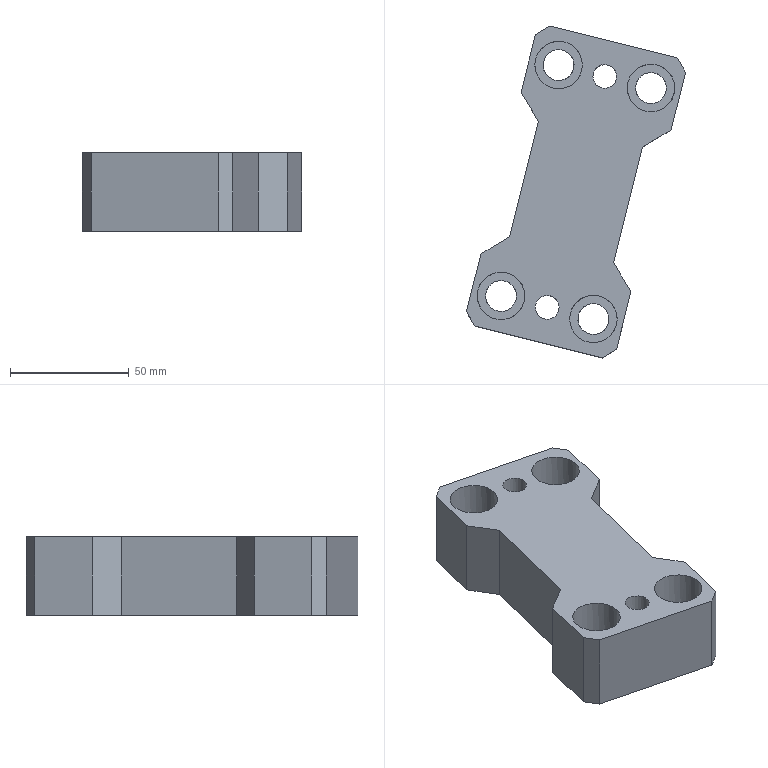Part | NX | features solid 2 | 1 solid | 32 faces | box 92.1 x 139.444 x 33 mm | volume 201833 mm3 | plane 22 | cylinder 10 | commonest cylinder face diameters 13 x4 20 x4 10 x2
STEP:
#1=CARTESIAN_POINT('',(-924.35,446.026,23.));
#2=VERTEX_POINT('',#1);
#3=CARTESIAN_POINT('',(-914.647,443.606,23.));
#4=DIRECTION('',(0.,0.,1.));
#5=DIRECTION('',(-0.9703,0.2419,0.));
#6=AXIS2_PLACEMENT_3D('',#3,#4,#5);
#7=CIRCLE('',#6,10.);
#8=EDGE_CURVE('',#2,#2,#7,.F.);
#9=ORIENTED_EDGE('',*,*,#8,.T.);
#10=EDGE_LOOP('',(#9));
#11=FACE_BOUND('',#10,.T.);
#12=CARTESIAN_POINT('',(-948.542,348.996,23.));
#13=VERTEX_POINT('',#12);
#14=CARTESIAN_POINT('',(-938.839,346.577,23.));
#15=DIRECTION('',(0.,0.,1.));
#16=DIRECTION('',(-0.9703,0.2419,0.));
#17=AXIS2_PLACEMENT_3D('',#14,#15,#16);
#18=CIRCLE('',#17,10.);
#19=EDGE_CURVE('',#13,#13,#18,.F.);
#20=ORIENTED_EDGE('',*,*,#19,.T.);
#21=EDGE_LOOP('',(#20));
#22=FACE_BOUND('',#21,.T.);
#23=CARTESIAN_POINT('',(-900.092,439.978,23.));
#24=VERTEX_POINT('',#23);
#25=CARTESIAN_POINT('',(-895.241,438.768,23.));
#26=DIRECTION('',(0.,0.,1.));
#27=DIRECTION('',(-0.9703,0.2419,0.));
#28=AXIS2_PLACEMENT_3D('',#25,#26,#27);
#29=CIRCLE('',#28,5.);
#30=EDGE_CURVE('',#24,#24,#29,.F.);
#31=ORIENTED_EDGE('',*,*,#30,.T.);
#32=EDGE_LOOP('',(#31));
#33=FACE_BOUND('',#32,.T.);
#34=CARTESIAN_POINT('',(-949.745,333.837,23.));
#35=VERTEX_POINT('',#34);
#36=CARTESIAN_POINT('',(-896.379,320.531,23.));
#37=VERTEX_POINT('',#36);
#38=CARTESIAN_POINT('',(-891.527,319.321,23.));
#39=DIRECTION('',(0.9703,-0.2419,0.));
#40=VECTOR('',#39,1000.);
#41=LINE('',#38,#40);
#42=EDGE_CURVE('',#35,#37,#41,.T.);
#43=ORIENTED_EDGE('',*,*,#42,.T.);
#44=CARTESIAN_POINT('',(-890.318,324.173,23.));
#45=VERTEX_POINT('',#44);
#46=CARTESIAN_POINT('',(-896.379,320.531,23.));
#47=DIRECTION('',(-0.8572,-0.515,0.));
#48=VECTOR('',#47,1000.);
#49=LINE('',#46,#48);
#50=EDGE_CURVE('',#45,#37,#49,.T.);
#51=ORIENTED_EDGE('',*,*,#50,.F.);
#52=CARTESIAN_POINT('',(-884.27,348.43,23.));
#53=VERTEX_POINT('',#52);
#54=CARTESIAN_POINT('',(-891.527,319.321,23.));
#55=DIRECTION('',(-0.2419,-0.9703,0.));
#56=VECTOR('',#55,1000.);
#57=LINE('',#54,#56);
#58=EDGE_CURVE('',#53,#45,#57,.T.);
#59=ORIENTED_EDGE('',*,*,#58,.F.);
#60=CARTESIAN_POINT('',(-891.553,360.553,23.));
#61=VERTEX_POINT('',#60);
#62=CARTESIAN_POINT('',(-873.344,330.247,23.));
#63=DIRECTION('',(0.515,-0.8572,0.));
#64=VECTOR('',#63,1000.);
#65=LINE('',#62,#64);
#66=EDGE_CURVE('',#61,#53,#65,.T.);
#67=ORIENTED_EDGE('',*,*,#66,.F.);
#68=CARTESIAN_POINT('',(-879.457,409.067,23.));
#69=VERTEX_POINT('',#68);
#70=CARTESIAN_POINT('',(-901.23,321.741,23.));
#71=DIRECTION('',(-0.2419,-0.9703,0.));
#72=VECTOR('',#71,1000.);
#73=LINE('',#70,#72);
#74=EDGE_CURVE('',#69,#61,#73,.T.);
#75=ORIENTED_EDGE('',*,*,#74,.F.);
#76=CARTESIAN_POINT('',(-867.335,416.351,23.));
#77=VERTEX_POINT('',#76);
#78=CARTESIAN_POINT('',(-927.946,379.932,23.));
#79=DIRECTION('',(0.8572,0.515,0.));
#80=VECTOR('',#79,1000.);
#81=LINE('',#78,#80);
#82=EDGE_CURVE('',#69,#77,#81,.T.);
#83=ORIENTED_EDGE('',*,*,#82,.T.);
#84=CARTESIAN_POINT('',(-861.287,440.608,23.));
#85=VERTEX_POINT('',#84);
#86=CARTESIAN_POINT('',(-891.527,319.321,23.));
#87=DIRECTION('',(-0.2419,-0.9703,0.));
#88=VECTOR('',#87,1000.);
#89=LINE('',#86,#88);
#90=EDGE_CURVE('',#85,#77,#89,.T.);
#91=ORIENTED_EDGE('',*,*,#90,.F.);
#92=CARTESIAN_POINT('',(-864.929,446.67,23.));
#93=VERTEX_POINT('',#92);
#94=CARTESIAN_POINT('',(-861.287,440.608,23.));
#95=DIRECTION('',(-0.515,0.8572,0.));
#96=VECTOR('',#95,1000.);
#97=LINE('',#94,#96);
#98=EDGE_CURVE('',#93,#85,#97,.F.);
#99=ORIENTED_EDGE('',*,*,#98,.F.);
#100=CARTESIAN_POINT('',(-918.295,459.975,23.));
#101=VERTEX_POINT('',#100);
#102=CARTESIAN_POINT('',(-860.077,445.46,23.));
#103=DIRECTION('',(0.9703,-0.2419,0.));
#104=VECTOR('',#103,1000.);
#105=LINE('',#102,#104);
#106=EDGE_CURVE('',#101,#93,#105,.T.);
#107=ORIENTED_EDGE('',*,*,#106,.F.);
#108=CARTESIAN_POINT('',(-924.356,456.333,23.));
#109=VERTEX_POINT('',#108);
#110=CARTESIAN_POINT('',(-918.295,459.975,23.));
#111=DIRECTION('',(0.8572,0.515,0.));
#112=VECTOR('',#111,1000.);
#113=LINE('',#110,#112);
#114=EDGE_CURVE('',#109,#101,#113,.T.);
#115=ORIENTED_EDGE('',*,*,#114,.F.);
#116=CARTESIAN_POINT('',(-930.404,432.076,23.));
#117=VERTEX_POINT('',#116);
#118=CARTESIAN_POINT('',(-954.596,335.046,23.));
#119=DIRECTION('',(-0.2419,-0.9703,0.));
#120=VECTOR('',#119,1000.);
#121=LINE('',#118,#120);
#122=EDGE_CURVE('',#109,#117,#121,.T.);
#123=ORIENTED_EDGE('',*,*,#122,.T.);
#124=CARTESIAN_POINT('',(-923.12,419.954,23.));
#125=VERTEX_POINT('',#124);
#126=CARTESIAN_POINT('',(-870.313,332.068,23.));
#127=DIRECTION('',(0.515,-0.8572,0.));
#128=VECTOR('',#127,1000.);
#129=LINE('',#126,#128);
#130=EDGE_CURVE('',#117,#125,#129,.T.);
#131=ORIENTED_EDGE('',*,*,#130,.T.);
#132=CARTESIAN_POINT('',(-935.217,371.439,23.));
#133=VERTEX_POINT('',#132);
#134=CARTESIAN_POINT('',(-944.893,332.627,23.));
#135=DIRECTION('',(-0.2419,-0.9703,0.));
#136=VECTOR('',#135,1000.);
#137=LINE('',#134,#136);
#138=EDGE_CURVE('',#125,#133,#137,.T.);
#139=ORIENTED_EDGE('',*,*,#138,.T.);
#140=CARTESIAN_POINT('',(-947.339,364.155,23.));
#141=VERTEX_POINT('',#140);
#142=CARTESIAN_POINT('',(-926.125,376.902,23.));
#143=DIRECTION('',(0.8572,0.515,0.));
#144=VECTOR('',#143,1000.);
#145=LINE('',#142,#144);
#146=EDGE_CURVE('',#141,#133,#145,.T.);
#147=ORIENTED_EDGE('',*,*,#146,.F.);
#148=CARTESIAN_POINT('',(-953.387,339.898,23.));
#149=VERTEX_POINT('',#148);
#150=CARTESIAN_POINT('',(-954.596,335.046,23.));
#151=DIRECTION('',(-0.2419,-0.9703,0.));
#152=VECTOR('',#151,1000.);
#153=LINE('',#150,#152);
#154=EDGE_CURVE('',#141,#149,#153,.T.);
#155=ORIENTED_EDGE('',*,*,#154,.T.);
#156=CARTESIAN_POINT('',(-953.387,339.898,23.));
#157=DIRECTION('',(0.515,-0.8572,0.));
#158=VECTOR('',#157,1000.);
#159=LINE('',#156,#158);
#160=EDGE_CURVE('',#35,#149,#159,.F.);
#161=ORIENTED_EDGE('',*,*,#160,.F.);
#162=EDGE_LOOP('',(#43,#51,#59,#67,#75,#83,#91,#99,#107,#115,#123,#131,#139,#147,#155,#161));
#163=FACE_BOUND('',#162,.T.);
#164=CARTESIAN_POINT('',(-924.284,342.948,23.));
#165=VERTEX_POINT('',#164);
#166=CARTESIAN_POINT('',(-919.433,341.738,23.));
#167=DIRECTION('',(0.,0.,1.));
#168=DIRECTION('',(-0.9703,0.2419,0.));
#169=AXIS2_PLACEMENT_3D('',#166,#167,#168);
#170=CIRCLE('',#169,5.);
#171=EDGE_CURVE('',#165,#165,#170,.F.);
#172=ORIENTED_EDGE('',*,*,#171,.T.);
#173=EDGE_LOOP('',(#172));
#174=FACE_BOUND('',#173,.T.);
#175=CARTESIAN_POINT('',(-909.73,339.319,23.));
#176=VERTEX_POINT('',#175);
#177=CARTESIAN_POINT('',(-900.027,336.9,23.));
#178=DIRECTION('',(0.,0.,1.));
#179=DIRECTION('',(-0.9703,0.2419,0.));
#180=AXIS2_PLACEMENT_3D('',#177,#178,#179);
#181=CIRCLE('',#180,10.);
#182=EDGE_CURVE('',#176,#176,#181,.F.);
#183=ORIENTED_EDGE('',*,*,#182,.T.);
#184=EDGE_LOOP('',(#183));
#185=FACE_BOUND('',#184,.T.);
#186=CARTESIAN_POINT('',(-885.538,436.349,23.));
#187=VERTEX_POINT('',#186);
#188=CARTESIAN_POINT('',(-875.835,433.93,23.));
#189=DIRECTION('',(0.,0.,1.));
#190=DIRECTION('',(-0.9703,0.2419,0.));
#191=AXIS2_PLACEMENT_3D('',#188,#189,#190);
#192=CIRCLE('',#191,10.);
#193=EDGE_CURVE('',#187,#187,#192,.F.);
#194=ORIENTED_EDGE('',*,*,#193,.T.);
#195=EDGE_LOOP('',(#194));
#196=FACE_BOUND('',#195,.T.);
#197=CARTESIAN_POINT('',(-891.527,319.321,23.));
#198=DIRECTION('',(0.,0.,-1.));
#199=DIRECTION('',(-0.9703,0.2419,0.));
#200=AXIS2_PLACEMENT_3D('',#197,#198,#199);
#201=PLANE('',#200);
#202=ADVANCED_FACE('',(#11,#22,#33,#163,#174,#185,#196),#201,.F.);
#203=CARTESIAN_POINT('',(-877.407,427.623,-10.));
#204=VERTEX_POINT('',#203);
#205=CARTESIAN_POINT('',(-875.835,433.93,-10.));
#206=DIRECTION('',(0.,0.,-1.));
#207=DIRECTION('',(-0.2419,-0.9703,0.));
#208=AXIS2_PLACEMENT_3D('',#205,#206,#207);
#209=CIRCLE('',#208,6.5);
#210=EDGE_CURVE('',#204,#204,#209,.T.);
#211=ORIENTED_EDGE('',*,*,#210,.T.);
#212=EDGE_LOOP('',(#211));
#213=FACE_BOUND('',#212,.T.);
#214=CARTESIAN_POINT('',(-869.528,432.357,5.));
#215=VERTEX_POINT('',#214);
#216=CARTESIAN_POINT('',(-875.835,433.93,5.));
#217=DIRECTION('',(0.,0.,-1.));
#218=DIRECTION('',(0.9703,-0.2419,0.));
#219=AXIS2_PLACEMENT_3D('',#216,#217,#218);
#220=CIRCLE('',#219,6.5);
#221=EDGE_CURVE('',#215,#215,#220,.T.);
#222=ORIENTED_EDGE('',*,*,#221,.F.);
#223=EDGE_LOOP('',(#222));
#224=FACE_BOUND('',#223,.T.);
#225=CARTESIAN_POINT('',(-875.835,433.93,12.));
#226=DIRECTION('',(0.,0.,-1.));
#227=DIRECTION('',(-0.9703,0.2419,0.));
#228=AXIS2_PLACEMENT_3D('',#225,#226,#227);
#229=CYLINDRICAL_SURFACE('',#228,6.5);
#230=ADVANCED_FACE('',(#213,#224),#229,.F.);
#231=CARTESIAN_POINT('',(-916.219,437.299,-10.));
#232=VERTEX_POINT('',#231);
#233=CARTESIAN_POINT('',(-914.647,443.606,-10.));
#234=DIRECTION('',(0.,0.,-1.));
#235=DIRECTION('',(-0.2419,-0.9703,0.));
#236=AXIS2_PLACEMENT_3D('',#233,#234,#235);
#237=CIRCLE('',#236,6.5);
#238=EDGE_CURVE('',#232,#232,#237,.T.);
#239=ORIENTED_EDGE('',*,*,#238,.T.);
#240=EDGE_LOOP('',(#239));
#241=FACE_BOUND('',#240,.T.);
#242=CARTESIAN_POINT('',(-908.34,442.034,5.));
#243=VERTEX_POINT('',#242);
#244=CARTESIAN_POINT('',(-914.647,443.606,5.));
#245=DIRECTION('',(0.,0.,-1.));
#246=DIRECTION('',(0.9703,-0.2419,0.));
#247=AXIS2_PLACEMENT_3D('',#244,#245,#246);
#248=CIRCLE('',#247,6.5);
#249=EDGE_CURVE('',#243,#243,#248,.T.);
#250=ORIENTED_EDGE('',*,*,#249,.F.);
#251=EDGE_LOOP('',(#250));
#252=FACE_BOUND('',#251,.T.);
#253=CARTESIAN_POINT('',(-914.647,443.606,12.));
#254=DIRECTION('',(0.,0.,-1.));
#255=DIRECTION('',(-0.9703,0.2419,0.));
#256=AXIS2_PLACEMENT_3D('',#253,#254,#255);
#257=CYLINDRICAL_SURFACE('',#256,6.5);
#258=ADVANCED_FACE('',(#241,#252),#257,.F.);
#259=CARTESIAN_POINT('',(-901.6,330.593,-10.));
#260=VERTEX_POINT('',#259);
#261=CARTESIAN_POINT('',(-900.027,336.9,-10.));
#262=DIRECTION('',(0.,0.,-1.));
#263=DIRECTION('',(-0.2419,-0.9703,0.));
#264=AXIS2_PLACEMENT_3D('',#261,#262,#263);
#265=CIRCLE('',#264,6.5);
#266=EDGE_CURVE('',#260,#260,#265,.T.);
#267=ORIENTED_EDGE('',*,*,#266,.T.);
#268=EDGE_LOOP('',(#267));
#269=FACE_BOUND('',#268,.T.);
#270=CARTESIAN_POINT('',(-893.72,335.327,5.));
#271=VERTEX_POINT('',#270);
#272=CARTESIAN_POINT('',(-900.027,336.9,5.));
#273=DIRECTION('',(0.,0.,-1.));
#274=DIRECTION('',(0.9703,-0.2419,0.));
#275=AXIS2_PLACEMENT_3D('',#272,#273,#274);
#276=CIRCLE('',#275,6.5);
#277=EDGE_CURVE('',#271,#271,#276,.T.);
#278=ORIENTED_EDGE('',*,*,#277,.F.);
#279=EDGE_LOOP('',(#278));
#280=FACE_BOUND('',#279,.T.);
#281=CARTESIAN_POINT('',(-900.027,336.9,12.));
#282=DIRECTION('',(0.,0.,-1.));
#283=DIRECTION('',(-0.9703,0.2419,0.));
#284=AXIS2_PLACEMENT_3D('',#281,#282,#283);
#285=CYLINDRICAL_SURFACE('',#284,6.5);
#286=ADVANCED_FACE('',(#269,#280),#285,.F.);
#287=CARTESIAN_POINT('',(-940.411,340.27,-10.));
#288=VERTEX_POINT('',#287);
#289=CARTESIAN_POINT('',(-938.839,346.577,-10.));
#290=DIRECTION('',(0.,0.,-1.));
#291=DIRECTION('',(-0.2419,-0.9703,0.));
#292=AXIS2_PLACEMENT_3D('',#289,#290,#291);
#293=CIRCLE('',#292,6.5);
#294=EDGE_CURVE('',#288,#288,#293,.T.);
#295=ORIENTED_EDGE('',*,*,#294,.T.);
#296=EDGE_LOOP('',(#295));
#297=FACE_BOUND('',#296,.T.);
#298=CARTESIAN_POINT('',(-932.532,345.004,5.));
#299=VERTEX_POINT('',#298);
#300=CARTESIAN_POINT('',(-938.839,346.577,5.));
#301=DIRECTION('',(0.,0.,-1.));
#302=DIRECTION('',(0.9703,-0.2419,0.));
#303=AXIS2_PLACEMENT_3D('',#300,#301,#302);
#304=CIRCLE('',#303,6.5);
#305=EDGE_CURVE('',#299,#299,#304,.T.);
#306=ORIENTED_EDGE('',*,*,#305,.F.);
#307=EDGE_LOOP('',(#306));
#308=FACE_BOUND('',#307,.T.);
#309=CARTESIAN_POINT('',(-938.839,346.577,12.));
#310=DIRECTION('',(0.,0.,-1.));
#311=DIRECTION('',(-0.9703,0.2419,0.));
#312=AXIS2_PLACEMENT_3D('',#309,#310,#311);
#313=CYLINDRICAL_SURFACE('',#312,6.5);
#314=ADVANCED_FACE('',(#297,#308),#313,.F.);
#315=CARTESIAN_POINT('',(-896.45,433.916,-10.));
#316=VERTEX_POINT('',#315);
#317=CARTESIAN_POINT('',(-895.241,438.768,-10.));
#318=DIRECTION('',(0.,0.,-1.));
#319=DIRECTION('',(-0.2419,-0.9703,0.));
#320=AXIS2_PLACEMENT_3D('',#317,#318,#319);
#321=CIRCLE('',#320,5.);
#322=EDGE_CURVE('',#316,#316,#321,.T.);
#323=ORIENTED_EDGE('',*,*,#322,.F.);
#324=EDGE_LOOP('',(#323));
#325=FACE_BOUND('',#324,.T.);
#326=ORIENTED_EDGE('',*,*,#266,.F.);
#327=EDGE_LOOP('',(#326));
#328=FACE_BOUND('',#327,.T.);
#329=ORIENTED_EDGE('',*,*,#294,.F.);
#330=EDGE_LOOP('',(#329));
#331=FACE_BOUND('',#330,.T.);
#332=CARTESIAN_POINT('',(-947.339,364.155,-10.));
#333=VERTEX_POINT('',#332);
#334=CARTESIAN_POINT('',(-953.387,339.898,-10.));
#335=VERTEX_POINT('',#334);
#336=CARTESIAN_POINT('',(-947.339,364.155,-10.));
#337=DIRECTION('',(-0.2419,-0.9703,0.));
#338=VECTOR('',#337,1000.);
#339=LINE('',#336,#338);
#340=EDGE_CURVE('',#333,#335,#339,.T.);
#341=ORIENTED_EDGE('',*,*,#340,.F.);
#342=CARTESIAN_POINT('',(-935.217,371.439,-10.));
#343=VERTEX_POINT('',#342);
#344=CARTESIAN_POINT('',(-947.339,364.155,-10.));
#345=DIRECTION('',(0.8572,0.515,0.));
#346=VECTOR('',#345,1000.);
#347=LINE('',#344,#346);
#348=EDGE_CURVE('',#333,#343,#347,.T.);
#349=ORIENTED_EDGE('',*,*,#348,.T.);
#350=CARTESIAN_POINT('',(-923.12,419.954,-10.));
#351=VERTEX_POINT('',#350);
#352=CARTESIAN_POINT('',(-923.12,419.954,-10.));
#353=DIRECTION('',(-0.2419,-0.9703,0.));
#354=VECTOR('',#353,1000.);
#355=LINE('',#352,#354);
#356=EDGE_CURVE('',#351,#343,#355,.T.);
#357=ORIENTED_EDGE('',*,*,#356,.F.);
#358=CARTESIAN_POINT('',(-930.404,432.076,-10.));
#359=VERTEX_POINT('',#358);
#360=CARTESIAN_POINT('',(-930.404,432.076,-10.));
#361=DIRECTION('',(0.515,-0.8572,0.));
#362=VECTOR('',#361,1000.);
#363=LINE('',#360,#362);
#364=EDGE_CURVE('',#359,#351,#363,.T.);
#365=ORIENTED_EDGE('',*,*,#364,.F.);
#366=CARTESIAN_POINT('',(-924.356,456.333,-10.));
#367=VERTEX_POINT('',#366);
#368=CARTESIAN_POINT('',(-923.147,461.185,-10.));
#369=DIRECTION('',(-0.2419,-0.9703,0.));
#370=VECTOR('',#369,1000.);
#371=LINE('',#368,#370);
#372=EDGE_CURVE('',#367,#359,#371,.T.);
#373=ORIENTED_EDGE('',*,*,#372,.F.);
#374=CARTESIAN_POINT('',(-918.295,459.975,-10.));
#375=VERTEX_POINT('',#374);
#376=CARTESIAN_POINT('',(-960.723,434.482,-10.));
#377=DIRECTION('',(-0.8572,-0.515,0.));
#378=VECTOR('',#377,1000.);
#379=LINE('',#376,#378);
#380=EDGE_CURVE('',#375,#367,#379,.T.);
#381=ORIENTED_EDGE('',*,*,#380,.F.);
#382=CARTESIAN_POINT('',(-864.929,446.67,-10.));
#383=VERTEX_POINT('',#382);
#384=CARTESIAN_POINT('',(-923.147,461.185,-10.));
#385=DIRECTION('',(0.9703,-0.2419,0.));
#386=VECTOR('',#385,1000.);
#387=LINE('',#384,#386);
#388=EDGE_CURVE('',#375,#383,#387,.T.);
#389=ORIENTED_EDGE('',*,*,#388,.T.);
#390=CARTESIAN_POINT('',(-861.287,440.608,-10.));
#391=VERTEX_POINT('',#390);
#392=CARTESIAN_POINT('',(-815.764,364.845,-10.));
#393=DIRECTION('',(0.515,-0.8572,0.));
#394=VECTOR('',#393,1000.);
#395=LINE('',#392,#394);
#396=EDGE_CURVE('',#391,#383,#395,.F.);
#397=ORIENTED_EDGE('',*,*,#396,.F.);
#398=CARTESIAN_POINT('',(-867.335,416.351,-10.));
#399=VERTEX_POINT('',#398);
#400=CARTESIAN_POINT('',(-860.077,445.46,-10.));
#401=DIRECTION('',(-0.2419,-0.9703,0.));
#402=VECTOR('',#401,1000.);
#403=LINE('',#400,#402);
#404=EDGE_CURVE('',#391,#399,#403,.T.);
#405=ORIENTED_EDGE('',*,*,#404,.T.);
#406=CARTESIAN_POINT('',(-879.457,409.067,-10.));
#407=VERTEX_POINT('',#406);
#408=CARTESIAN_POINT('',(-879.457,409.067,-10.));
#409=DIRECTION('',(0.8572,0.515,0.));
#410=VECTOR('',#409,1000.);
#411=LINE('',#408,#410);
#412=EDGE_CURVE('',#407,#399,#411,.T.);
#413=ORIENTED_EDGE('',*,*,#412,.F.);
#414=CARTESIAN_POINT('',(-891.553,360.553,-10.));
#415=VERTEX_POINT('',#414);
#416=CARTESIAN_POINT('',(-879.457,409.067,-10.));
#417=DIRECTION('',(-0.2419,-0.9703,0.));
#418=VECTOR('',#417,1000.);
#419=LINE('',#416,#418);
#420=EDGE_CURVE('',#407,#415,#419,.T.);
#421=ORIENTED_EDGE('',*,*,#420,.T.);
#422=CARTESIAN_POINT('',(-884.27,348.43,-10.));
#423=VERTEX_POINT('',#422);
#424=CARTESIAN_POINT('',(-891.553,360.553,-10.));
#425=DIRECTION('',(0.515,-0.8572,0.));
#426=VECTOR('',#425,1000.);
#427=LINE('',#424,#426);
#428=EDGE_CURVE('',#415,#423,#427,.T.);
#429=ORIENTED_EDGE('',*,*,#428,.T.);
#430=CARTESIAN_POINT('',(-890.318,324.173,-10.));
#431=VERTEX_POINT('',#430);
#432=CARTESIAN_POINT('',(-884.27,348.43,-10.));
#433=DIRECTION('',(-0.2419,-0.9703,0.));
#434=VECTOR('',#433,1000.);
#435=LINE('',#432,#434);
#436=EDGE_CURVE('',#423,#431,#435,.T.);
#437=ORIENTED_EDGE('',*,*,#436,.T.);
#438=CARTESIAN_POINT('',(-896.379,320.531,-10.));
#439=VERTEX_POINT('',#438);
#440=CARTESIAN_POINT('',(-893.348,322.352,-10.));
#441=DIRECTION('',(0.8572,0.515,0.));
#442=VECTOR('',#441,1000.);
#443=LINE('',#440,#442);
#444=EDGE_CURVE('',#439,#431,#443,.T.);
#445=ORIENTED_EDGE('',*,*,#444,.F.);
#446=CARTESIAN_POINT('',(-949.745,333.837,-10.));
#447=VERTEX_POINT('',#446);
#448=CARTESIAN_POINT('',(-954.596,335.046,-10.));
#449=DIRECTION('',(0.9703,-0.2419,0.));
#450=VECTOR('',#449,1000.);
#451=LINE('',#448,#450);
#452=EDGE_CURVE('',#447,#439,#451,.T.);
#453=ORIENTED_EDGE('',*,*,#452,.F.);
#454=CARTESIAN_POINT('',(-927.894,297.47,-10.));
#455=DIRECTION('',(-0.515,0.8572,0.));
#456=VECTOR('',#455,1000.);
#457=LINE('',#454,#456);
#458=EDGE_CURVE('',#335,#447,#457,.F.);
#459=ORIENTED_EDGE('',*,*,#458,.F.);
#460=EDGE_LOOP('',(#341,#349,#357,#365,#373,#381,#389,#397,#405,#413,#421,#429,#437,#445,#453,#459));
#461=FACE_BOUND('',#460,.T.);
#462=CARTESIAN_POINT('',(-920.643,336.887,-10.));
#463=VERTEX_POINT('',#462);
#464=CARTESIAN_POINT('',(-919.433,341.738,-10.));
#465=DIRECTION('',(0.,0.,-1.));
#466=DIRECTION('',(-0.2419,-0.9703,0.));
#467=AXIS2_PLACEMENT_3D('',#464,#465,#466);
#468=CIRCLE('',#467,5.);
#469=EDGE_CURVE('',#463,#463,#468,.T.);
#470=ORIENTED_EDGE('',*,*,#469,.F.);
#471=EDGE_LOOP('',(#470));
#472=FACE_BOUND('',#471,.T.);
#473=ORIENTED_EDGE('',*,*,#238,.F.);
#474=EDGE_LOOP('',(#473));
#475=FACE_BOUND('',#474,.T.);
#476=ORIENTED_EDGE('',*,*,#210,.F.);
#477=EDGE_LOOP('',(#476));
#478=FACE_BOUND('',#477,.T.);
#479=CARTESIAN_POINT('',(-891.527,319.321,-10.));
#480=DIRECTION('',(0.,0.,-1.));
#481=DIRECTION('',(-0.9703,0.2419,0.));
#482=AXIS2_PLACEMENT_3D('',#479,#480,#481);
#483=PLANE('',#482);
#484=ADVANCED_FACE('',(#325,#328,#331,#461,#472,#475,#478),#483,.T.);
#485=ORIENTED_EDGE('',*,*,#90,.T.);
#486=CARTESIAN_POINT('',(-867.335,416.351,12.));
#487=DIRECTION('',(0.,0.,-1.));
#488=VECTOR('',#487,1000.);
#489=LINE('',#486,#488);
#490=EDGE_CURVE('',#77,#399,#489,.T.);
#491=ORIENTED_EDGE('',*,*,#490,.T.);
#492=ORIENTED_EDGE('',*,*,#404,.F.);
#493=CARTESIAN_POINT('',(-861.287,440.608,12.));
#494=DIRECTION('',(0.,0.,-1.));
#495=VECTOR('',#494,1000.);
#496=LINE('',#493,#495);
#497=EDGE_CURVE('',#85,#391,#496,.T.);
#498=ORIENTED_EDGE('',*,*,#497,.F.);
#499=EDGE_LOOP('',(#485,#491,#492,#498));
#500=FACE_BOUND('',#499,.T.);
#501=CARTESIAN_POINT('',(-860.077,445.46,12.));
#502=DIRECTION('',(-0.9703,0.2419,0.));
#503=DIRECTION('',(0.2419,0.9703,0.));
#504=AXIS2_PLACEMENT_3D('',#501,#502,#503);
#505=PLANE('',#504);
#506=ADVANCED_FACE('',(#500),#505,.F.);
#507=ORIENTED_EDGE('',*,*,#412,.T.);
#508=ORIENTED_EDGE('',*,*,#490,.F.);
#509=ORIENTED_EDGE('',*,*,#82,.F.);
#510=CARTESIAN_POINT('',(-879.457,409.067,12.));
#511=DIRECTION('',(0.,0.,-1.));
#512=VECTOR('',#511,1000.);
#513=LINE('',#510,#512);
#514=EDGE_CURVE('',#69,#407,#513,.T.);
#515=ORIENTED_EDGE('',*,*,#514,.T.);
#516=EDGE_LOOP('',(#507,#508,#509,#515));
#517=FACE_BOUND('',#516,.T.);
#518=CARTESIAN_POINT('',(-879.457,409.067,12.));
#519=DIRECTION('',(0.515,-0.8572,0.));
#520=DIRECTION('',(-0.8572,-0.515,0.));
#521=AXIS2_PLACEMENT_3D('',#518,#519,#520);
#522=PLANE('',#521);
#523=ADVANCED_FACE('',(#517),#522,.T.);
#524=ORIENTED_EDGE('',*,*,#420,.F.);
#525=ORIENTED_EDGE('',*,*,#514,.F.);
#526=ORIENTED_EDGE('',*,*,#74,.T.);
#527=CARTESIAN_POINT('',(-891.553,360.553,12.));
#528=DIRECTION('',(0.,0.,-1.));
#529=VECTOR('',#528,1000.);
#530=LINE('',#527,#529);
#531=EDGE_CURVE('',#61,#415,#530,.T.);
#532=ORIENTED_EDGE('',*,*,#531,.T.);
#533=EDGE_LOOP('',(#524,#525,#526,#532));
#534=FACE_BOUND('',#533,.T.);
#535=CARTESIAN_POINT('',(-879.457,409.067,12.));
#536=DIRECTION('',(-0.9703,0.2419,0.));
#537=DIRECTION('',(0.2419,0.9703,0.));
#538=AXIS2_PLACEMENT_3D('',#535,#536,#537);
#539=PLANE('',#538);
#540=ADVANCED_FACE('',(#534),#539,.F.);
#541=ORIENTED_EDGE('',*,*,#428,.F.);
#542=ORIENTED_EDGE('',*,*,#531,.F.);
#543=ORIENTED_EDGE('',*,*,#66,.T.);
#544=CARTESIAN_POINT('',(-884.27,348.43,12.));
#545=DIRECTION('',(0.,0.,-1.));
#546=VECTOR('',#545,1000.);
#547=LINE('',#544,#546);
#548=EDGE_CURVE('',#53,#423,#547,.T.);
#549=ORIENTED_EDGE('',*,*,#548,.T.);
#550=EDGE_LOOP('',(#541,#542,#543,#549));
#551=FACE_BOUND('',#550,.T.);
#552=CARTESIAN_POINT('',(-891.553,360.553,12.));
#553=DIRECTION('',(-0.8572,-0.515,0.));
#554=DIRECTION('',(-0.515,0.8572,0.));
#555=AXIS2_PLACEMENT_3D('',#552,#553,#554);
#556=PLANE('',#555);
#557=ADVANCED_FACE('',(#551),#556,.F.);
#558=ORIENTED_EDGE('',*,*,#436,.F.);
#559=ORIENTED_EDGE('',*,*,#548,.F.);
#560=ORIENTED_EDGE('',*,*,#58,.T.);
#561=CARTESIAN_POINT('',(-890.318,324.173,23.));
#562=DIRECTION('',(0.,0.,1.));
#563=VECTOR('',#562,1000.);
#564=LINE('',#561,#563);
#565=EDGE_CURVE('',#431,#45,#564,.T.);
#566=ORIENTED_EDGE('',*,*,#565,.F.);
#567=EDGE_LOOP('',(#558,#559,#560,#566));
#568=FACE_BOUND('',#567,.T.);
#569=CARTESIAN_POINT('',(-884.27,348.43,12.));
#570=DIRECTION('',(-0.9703,0.2419,0.));
#571=DIRECTION('',(0.2419,0.9703,0.));
#572=AXIS2_PLACEMENT_3D('',#569,#570,#571);
#573=PLANE('',#572);
#574=ADVANCED_FACE('',(#568),#573,.F.);
#575=ORIENTED_EDGE('',*,*,#452,.T.);
#576=CARTESIAN_POINT('',(-896.379,320.531,-10.));
#577=DIRECTION('',(0.,0.,-1.));
#578=VECTOR('',#577,1000.);
#579=LINE('',#576,#578);
#580=EDGE_CURVE('',#37,#439,#579,.T.);
#581=ORIENTED_EDGE('',*,*,#580,.F.);
#582=ORIENTED_EDGE('',*,*,#42,.F.);
#583=CARTESIAN_POINT('',(-949.745,333.837,12.));
#584=DIRECTION('',(0.,0.,1.));
#585=VECTOR('',#584,1000.);
#586=LINE('',#583,#585);
#587=EDGE_CURVE('',#447,#35,#586,.T.);
#588=ORIENTED_EDGE('',*,*,#587,.F.);
#589=EDGE_LOOP('',(#575,#581,#582,#588));
#590=FACE_BOUND('',#589,.T.);
#591=CARTESIAN_POINT('',(-954.596,335.046,12.));
#592=DIRECTION('',(-0.2419,-0.9703,0.));
#593=DIRECTION('',(-0.9703,0.2419,0.));
#594=AXIS2_PLACEMENT_3D('',#591,#592,#593);
#595=PLANE('',#594);
#596=ADVANCED_FACE('',(#590),#595,.T.);
#597=ORIENTED_EDGE('',*,*,#154,.F.);
#598=CARTESIAN_POINT('',(-947.339,364.155,12.));
#599=DIRECTION('',(0.,0.,-1.));
#600=VECTOR('',#599,1000.);
#601=LINE('',#598,#600);
#602=EDGE_CURVE('',#141,#333,#601,.T.);
#603=ORIENTED_EDGE('',*,*,#602,.T.);
#604=ORIENTED_EDGE('',*,*,#340,.T.);
#605=CARTESIAN_POINT('',(-953.387,339.898,12.));
#606=DIRECTION('',(0.,0.,-1.));
#607=VECTOR('',#606,1000.);
#608=LINE('',#605,#607);
#609=EDGE_CURVE('',#149,#335,#608,.T.);
#610=ORIENTED_EDGE('',*,*,#609,.F.);
#611=EDGE_LOOP('',(#597,#603,#604,#610));
#612=FACE_BOUND('',#611,.T.);
#613=CARTESIAN_POINT('',(-947.339,364.155,12.));
#614=DIRECTION('',(-0.9703,0.2419,0.));
#615=DIRECTION('',(0.2419,0.9703,0.));
#616=AXIS2_PLACEMENT_3D('',#613,#614,#615);
#617=PLANE('',#616);
#618=ADVANCED_FACE('',(#612),#617,.T.);
#619=ORIENTED_EDGE('',*,*,#348,.F.);
#620=ORIENTED_EDGE('',*,*,#602,.F.);
#621=ORIENTED_EDGE('',*,*,#146,.T.);
#622=CARTESIAN_POINT('',(-935.217,371.439,12.));
#623=DIRECTION('',(0.,0.,-1.));
#624=VECTOR('',#623,1000.);
#625=LINE('',#622,#624);
#626=EDGE_CURVE('',#133,#343,#625,.T.);
#627=ORIENTED_EDGE('',*,*,#626,.T.);
#628=EDGE_LOOP('',(#619,#620,#621,#627));
#629=FACE_BOUND('',#628,.T.);
#630=CARTESIAN_POINT('',(-947.339,364.155,12.));
#631=DIRECTION('',(0.515,-0.8572,0.));
#632=DIRECTION('',(-0.8572,-0.515,0.));
#633=AXIS2_PLACEMENT_3D('',#630,#631,#632);
#634=PLANE('',#633);
#635=ADVANCED_FACE('',(#629),#634,.F.);
#636=ORIENTED_EDGE('',*,*,#356,.T.);
#637=ORIENTED_EDGE('',*,*,#626,.F.);
#638=ORIENTED_EDGE('',*,*,#138,.F.);
#639=CARTESIAN_POINT('',(-923.12,419.954,12.));
#640=DIRECTION('',(0.,0.,-1.));
#641=VECTOR('',#640,1000.);
#642=LINE('',#639,#641);
#643=EDGE_CURVE('',#125,#351,#642,.T.);
#644=ORIENTED_EDGE('',*,*,#643,.T.);
#645=EDGE_LOOP('',(#636,#637,#638,#644));
#646=FACE_BOUND('',#645,.T.);
#647=CARTESIAN_POINT('',(-923.12,419.954,12.));
#648=DIRECTION('',(-0.9703,0.2419,0.));
#649=DIRECTION('',(0.2419,0.9703,0.));
#650=AXIS2_PLACEMENT_3D('',#647,#648,#649);
#651=PLANE('',#650);
#652=ADVANCED_FACE('',(#646),#651,.T.);
#653=ORIENTED_EDGE('',*,*,#364,.T.);
#654=ORIENTED_EDGE('',*,*,#643,.F.);
#655=ORIENTED_EDGE('',*,*,#130,.F.);
#656=CARTESIAN_POINT('',(-930.404,432.076,12.));
#657=DIRECTION('',(0.,0.,-1.));
#658=VECTOR('',#657,1000.);
#659=LINE('',#656,#658);
#660=EDGE_CURVE('',#117,#359,#659,.T.);
#661=ORIENTED_EDGE('',*,*,#660,.T.);
#662=EDGE_LOOP('',(#653,#654,#655,#661));
#663=FACE_BOUND('',#662,.T.);
#664=CARTESIAN_POINT('',(-930.404,432.076,12.));
#665=DIRECTION('',(-0.8572,-0.515,0.));
#666=DIRECTION('',(-0.515,0.8572,0.));
#667=AXIS2_PLACEMENT_3D('',#664,#665,#666);
#668=PLANE('',#667);
#669=ADVANCED_FACE('',(#663),#668,.T.);
#670=ORIENTED_EDGE('',*,*,#372,.T.);
#671=ORIENTED_EDGE('',*,*,#660,.F.);
#672=ORIENTED_EDGE('',*,*,#122,.F.);
#673=CARTESIAN_POINT('',(-924.356,456.333,23.));
#674=DIRECTION('',(0.,0.,1.));
#675=VECTOR('',#674,1000.);
#676=LINE('',#673,#675);
#677=EDGE_CURVE('',#367,#109,#676,.T.);
#678=ORIENTED_EDGE('',*,*,#677,.F.);
#679=EDGE_LOOP('',(#670,#671,#672,#678));
#680=FACE_BOUND('',#679,.T.);
#681=CARTESIAN_POINT('',(-923.147,461.185,12.));
#682=DIRECTION('',(-0.9703,0.2419,0.));
#683=DIRECTION('',(0.2419,0.9703,0.));
#684=AXIS2_PLACEMENT_3D('',#681,#682,#683);
#685=PLANE('',#684);
#686=ADVANCED_FACE('',(#680),#685,.T.);
#687=ORIENTED_EDGE('',*,*,#106,.T.);
#688=CARTESIAN_POINT('',(-864.929,446.67,12.));
#689=DIRECTION('',(0.,0.,1.));
#690=VECTOR('',#689,1000.);
#691=LINE('',#688,#690);
#692=EDGE_CURVE('',#383,#93,#691,.T.);
#693=ORIENTED_EDGE('',*,*,#692,.F.);
#694=ORIENTED_EDGE('',*,*,#388,.F.);
#695=CARTESIAN_POINT('',(-918.295,459.975,-10.));
#696=DIRECTION('',(0.,0.,-1.));
#697=VECTOR('',#696,1000.);
#698=LINE('',#695,#697);
#699=EDGE_CURVE('',#101,#375,#698,.T.);
#700=ORIENTED_EDGE('',*,*,#699,.F.);
#701=EDGE_LOOP('',(#687,#693,#694,#700));
#702=FACE_BOUND('',#701,.T.);
#703=CARTESIAN_POINT('',(-923.147,461.185,12.));
#704=DIRECTION('',(-0.2419,-0.9703,0.));
#705=DIRECTION('',(-0.9703,0.2419,0.));
#706=AXIS2_PLACEMENT_3D('',#703,#704,#705);
#707=PLANE('',#706);
#708=ADVANCED_FACE('',(#702),#707,.F.);
#709=ORIENTED_EDGE('',*,*,#171,.F.);
#710=EDGE_LOOP('',(#709));
#711=FACE_BOUND('',#710,.T.);
#712=ORIENTED_EDGE('',*,*,#469,.T.);
#713=EDGE_LOOP('',(#712));
#714=FACE_BOUND('',#713,.T.);
#715=CARTESIAN_POINT('',(-919.433,341.738,12.));
#716=DIRECTION('',(0.,0.,-1.));
#717=DIRECTION('',(-0.9703,0.2419,0.));
#718=AXIS2_PLACEMENT_3D('',#715,#716,#717);
#719=CYLINDRICAL_SURFACE('',#718,5.);
#720=ADVANCED_FACE('',(#711,#714),#719,.F.);
#721=ORIENTED_EDGE('',*,*,#30,.F.);
#722=EDGE_LOOP('',(#721));
#723=FACE_BOUND('',#722,.T.);
#724=ORIENTED_EDGE('',*,*,#322,.T.);
#725=EDGE_LOOP('',(#724));
#726=FACE_BOUND('',#725,.T.);
#727=CARTESIAN_POINT('',(-895.241,438.768,12.));
#728=DIRECTION('',(0.,0.,-1.));
#729=DIRECTION('',(-0.9703,0.2419,0.));
#730=AXIS2_PLACEMENT_3D('',#727,#728,#729);
#731=CYLINDRICAL_SURFACE('',#730,5.);
#732=ADVANCED_FACE('',(#723,#726),#731,.F.);
#733=ORIENTED_EDGE('',*,*,#19,.F.);
#734=EDGE_LOOP('',(#733));
#735=FACE_BOUND('',#734,.T.);
#736=CARTESIAN_POINT('',(-941.258,336.874,5.));
#737=VERTEX_POINT('',#736);
#738=CARTESIAN_POINT('',(-938.839,346.577,5.));
#739=DIRECTION('',(0.,0.,-1.));
#740=DIRECTION('',(-0.2419,-0.9703,0.));
#741=AXIS2_PLACEMENT_3D('',#738,#739,#740);
#742=CIRCLE('',#741,10.);
#743=EDGE_CURVE('',#737,#737,#742,.T.);
#744=ORIENTED_EDGE('',*,*,#743,.T.);
#745=EDGE_LOOP('',(#744));
#746=FACE_BOUND('',#745,.T.);
#747=CARTESIAN_POINT('',(-938.839,346.577,12.));
#748=DIRECTION('',(0.,0.,-1.));
#749=DIRECTION('',(-0.9703,0.2419,0.));
#750=AXIS2_PLACEMENT_3D('',#747,#748,#749);
#751=CYLINDRICAL_SURFACE('',#750,10.);
#752=ADVANCED_FACE('',(#735,#746),#751,.F.);
#753=ORIENTED_EDGE('',*,*,#305,.T.);
#754=EDGE_LOOP('',(#753));
#755=FACE_BOUND('',#754,.T.);
#756=ORIENTED_EDGE('',*,*,#743,.F.);
#757=EDGE_LOOP('',(#756));
#758=FACE_BOUND('',#757,.T.);
#759=CARTESIAN_POINT('',(-938.839,346.577,5.));
#760=DIRECTION('',(0.,0.,1.));
#761=DIRECTION('',(0.9703,-0.2419,0.));
#762=AXIS2_PLACEMENT_3D('',#759,#760,#761);
#763=PLANE('',#762);
#764=ADVANCED_FACE('',(#755,#758),#763,.T.);
#765=ORIENTED_EDGE('',*,*,#182,.F.);
#766=EDGE_LOOP('',(#765));
#767=FACE_BOUND('',#766,.T.);
#768=CARTESIAN_POINT('',(-902.446,327.197,5.));
#769=VERTEX_POINT('',#768);
#770=CARTESIAN_POINT('',(-900.027,336.9,5.));
#771=DIRECTION('',(0.,0.,-1.));
#772=DIRECTION('',(-0.2419,-0.9703,0.));
#773=AXIS2_PLACEMENT_3D('',#770,#771,#772);
#774=CIRCLE('',#773,10.);
#775=EDGE_CURVE('',#769,#769,#774,.T.);
#776=ORIENTED_EDGE('',*,*,#775,.T.);
#777=EDGE_LOOP('',(#776));
#778=FACE_BOUND('',#777,.T.);
#779=CARTESIAN_POINT('',(-900.027,336.9,12.));
#780=DIRECTION('',(0.,0.,-1.));
#781=DIRECTION('',(-0.9703,0.2419,0.));
#782=AXIS2_PLACEMENT_3D('',#779,#780,#781);
#783=CYLINDRICAL_SURFACE('',#782,10.);
#784=ADVANCED_FACE('',(#767,#778),#783,.F.);
#785=ORIENTED_EDGE('',*,*,#277,.T.);
#786=EDGE_LOOP('',(#785));
#787=FACE_BOUND('',#786,.T.);
#788=ORIENTED_EDGE('',*,*,#775,.F.);
#789=EDGE_LOOP('',(#788));
#790=FACE_BOUND('',#789,.T.);
#791=CARTESIAN_POINT('',(-900.027,336.9,5.));
#792=DIRECTION('',(0.,0.,1.));
#793=DIRECTION('',(0.9703,-0.2419,0.));
#794=AXIS2_PLACEMENT_3D('',#791,#792,#793);
#795=PLANE('',#794);
#796=ADVANCED_FACE('',(#787,#790),#795,.T.);
#797=ORIENTED_EDGE('',*,*,#8,.F.);
#798=EDGE_LOOP('',(#797));
#799=FACE_BOUND('',#798,.T.);
#800=CARTESIAN_POINT('',(-917.066,433.903,5.));
#801=VERTEX_POINT('',#800);
#802=CARTESIAN_POINT('',(-914.647,443.606,5.));
#803=DIRECTION('',(0.,0.,-1.));
#804=DIRECTION('',(-0.2419,-0.9703,0.));
#805=AXIS2_PLACEMENT_3D('',#802,#803,#804);
#806=CIRCLE('',#805,10.);
#807=EDGE_CURVE('',#801,#801,#806,.T.);
#808=ORIENTED_EDGE('',*,*,#807,.T.);
#809=EDGE_LOOP('',(#808));
#810=FACE_BOUND('',#809,.T.);
#811=CARTESIAN_POINT('',(-914.647,443.606,12.));
#812=DIRECTION('',(0.,0.,-1.));
#813=DIRECTION('',(-0.9703,0.2419,0.));
#814=AXIS2_PLACEMENT_3D('',#811,#812,#813);
#815=CYLINDRICAL_SURFACE('',#814,10.);
#816=ADVANCED_FACE('',(#799,#810),#815,.F.);
#817=ORIENTED_EDGE('',*,*,#249,.T.);
#818=EDGE_LOOP('',(#817));
#819=FACE_BOUND('',#818,.T.);
#820=ORIENTED_EDGE('',*,*,#807,.F.);
#821=EDGE_LOOP('',(#820));
#822=FACE_BOUND('',#821,.T.);
#823=CARTESIAN_POINT('',(-914.647,443.606,5.));
#824=DIRECTION('',(0.,0.,1.));
#825=DIRECTION('',(0.9703,-0.2419,0.));
#826=AXIS2_PLACEMENT_3D('',#823,#824,#825);
#827=PLANE('',#826);
#828=ADVANCED_FACE('',(#819,#822),#827,.T.);
#829=ORIENTED_EDGE('',*,*,#193,.F.);
#830=EDGE_LOOP('',(#829));
#831=FACE_BOUND('',#830,.T.);
#832=CARTESIAN_POINT('',(-878.254,424.227,5.));
#833=VERTEX_POINT('',#832);
#834=CARTESIAN_POINT('',(-875.835,433.93,5.));
#835=DIRECTION('',(0.,0.,-1.));
#836=DIRECTION('',(-0.2419,-0.9703,0.));
#837=AXIS2_PLACEMENT_3D('',#834,#835,#836);
#838=CIRCLE('',#837,10.);
#839=EDGE_CURVE('',#833,#833,#838,.T.);
#840=ORIENTED_EDGE('',*,*,#839,.T.);
#841=EDGE_LOOP('',(#840));
#842=FACE_BOUND('',#841,.T.);
#843=CARTESIAN_POINT('',(-875.835,433.93,12.));
#844=DIRECTION('',(0.,0.,-1.));
#845=DIRECTION('',(-0.9703,0.2419,0.));
#846=AXIS2_PLACEMENT_3D('',#843,#844,#845);
#847=CYLINDRICAL_SURFACE('',#846,10.);
#848=ADVANCED_FACE('',(#831,#842),#847,.F.);
#849=ORIENTED_EDGE('',*,*,#221,.T.);
#850=EDGE_LOOP('',(#849));
#851=FACE_BOUND('',#850,.T.);
#852=ORIENTED_EDGE('',*,*,#839,.F.);
#853=EDGE_LOOP('',(#852));
#854=FACE_BOUND('',#853,.T.);
#855=CARTESIAN_POINT('',(-875.835,433.93,5.));
#856=DIRECTION('',(0.,0.,1.));
#857=DIRECTION('',(0.9703,-0.2419,0.));
#858=AXIS2_PLACEMENT_3D('',#855,#856,#857);
#859=PLANE('',#858);
#860=ADVANCED_FACE('',(#851,#854),#859,.T.);
#861=ORIENTED_EDGE('',*,*,#160,.T.);
#862=ORIENTED_EDGE('',*,*,#609,.T.);
#863=ORIENTED_EDGE('',*,*,#458,.T.);
#864=ORIENTED_EDGE('',*,*,#587,.T.);
#865=EDGE_LOOP('',(#861,#862,#863,#864));
#866=FACE_BOUND('',#865,.T.);
#867=CARTESIAN_POINT('',(-953.387,339.898,12.));
#868=DIRECTION('',(0.8572,0.515,0.));
#869=DIRECTION('',(0.515,-0.8572,0.));
#870=AXIS2_PLACEMENT_3D('',#867,#868,#869);
#871=PLANE('',#870);
#872=ADVANCED_FACE('',(#866),#871,.F.);
#873=ORIENTED_EDGE('',*,*,#50,.T.);
#874=ORIENTED_EDGE('',*,*,#580,.T.);
#875=ORIENTED_EDGE('',*,*,#444,.T.);
#876=ORIENTED_EDGE('',*,*,#565,.T.);
#877=EDGE_LOOP('',(#873,#874,#875,#876));
#878=FACE_BOUND('',#877,.T.);
#879=CARTESIAN_POINT('',(-896.379,320.531,12.));
#880=DIRECTION('',(0.515,-0.8572,0.));
#881=DIRECTION('',(-0.8572,-0.515,0.));
#882=AXIS2_PLACEMENT_3D('',#879,#880,#881);
#883=PLANE('',#882);
#884=ADVANCED_FACE('',(#878),#883,.T.);
#885=ORIENTED_EDGE('',*,*,#114,.T.);
#886=ORIENTED_EDGE('',*,*,#699,.T.);
#887=ORIENTED_EDGE('',*,*,#380,.T.);
#888=ORIENTED_EDGE('',*,*,#677,.T.);
#889=EDGE_LOOP('',(#885,#886,#887,#888));
#890=FACE_BOUND('',#889,.T.);
#891=CARTESIAN_POINT('',(-918.295,459.975,12.));
#892=DIRECTION('',(-0.515,0.8572,0.));
#893=DIRECTION('',(0.8572,0.515,0.));
#894=AXIS2_PLACEMENT_3D('',#891,#892,#893);
#895=PLANE('',#894);
#896=ADVANCED_FACE('',(#890),#895,.T.);
#897=ORIENTED_EDGE('',*,*,#98,.T.);
#898=ORIENTED_EDGE('',*,*,#497,.T.);
#899=ORIENTED_EDGE('',*,*,#396,.T.);
#900=ORIENTED_EDGE('',*,*,#692,.T.);
#901=EDGE_LOOP('',(#897,#898,#899,#900));
#902=FACE_BOUND('',#901,.T.);
#903=CARTESIAN_POINT('',(-861.287,440.608,12.));
#904=DIRECTION('',(-0.8572,-0.515,0.));
#905=DIRECTION('',(-0.515,0.8572,0.));
#906=AXIS2_PLACEMENT_3D('',#903,#904,#905);
#907=PLANE('',#906);
#908=ADVANCED_FACE('',(#902),#907,.F.);
#909=CLOSED_SHELL('',(#202,#230,#258,#286,#314,#484,#506,#523,#540,#557,#574,#596,#618,#635,#652,#669,#686,#708,#720,#732,#752,#764,#784,#796,#816,#828,#848,#860,#872,#884,#896,#908));
#910=MANIFOLD_SOLID_BREP('',#909);
#911=(LENGTH_UNIT()NAMED_UNIT(*)SI_UNIT(.MILLI.,.METRE.));
#912=UNCERTAINTY_MEASURE_WITH_UNIT(LENGTH_MEASURE(0.00001),#911,'','');
#913=(NAMED_UNIT(*)PLANE_ANGLE_UNIT()SI_UNIT($,.RADIAN.));
#914=(NAMED_UNIT(*)SI_UNIT($,.STERADIAN.)SOLID_ANGLE_UNIT());
#915=(GEOMETRIC_REPRESENTATION_CONTEXT(3)GLOBAL_UNCERTAINTY_ASSIGNED_CONTEXT((#912))GLOBAL_UNIT_ASSIGNED_CONTEXT((#911,#913,#914))REPRESENTATION_CONTEXT('',''));
#916=ADVANCED_BREP_SHAPE_REPRESENTATION('',(#910),#915);